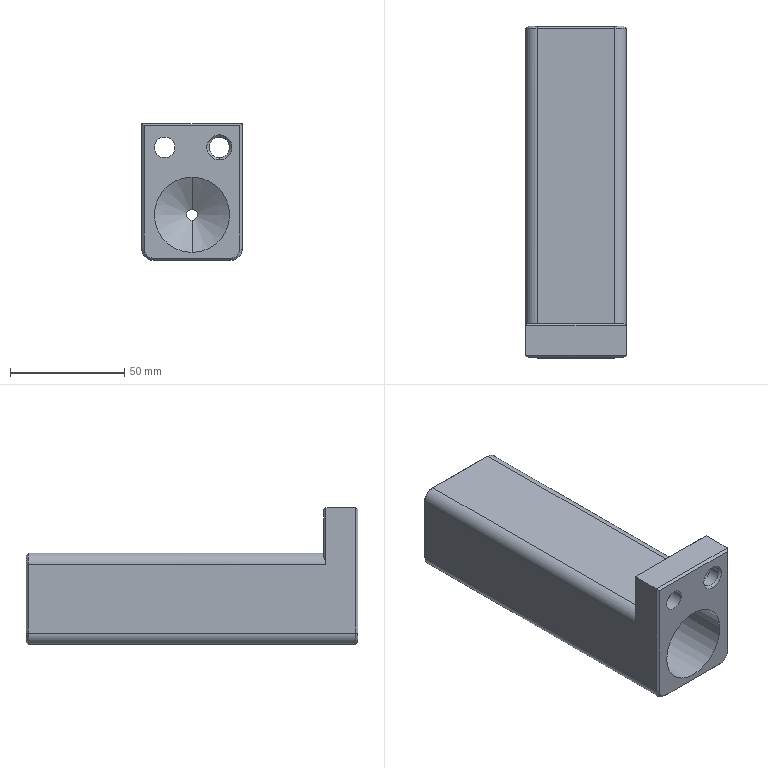Part | Creo | 1 solid | 45 faces | box 44 x 145.5 x 60 mm | volume 142551 mm3 | plane 21 | cylinder 14 | cone 10 | commonest cylinder face diameters 9 x4 10 x4 14 x4 33 x2
STEP:
#1=CARTESIAN_POINT('',(0.,0.,0.));
#2=DIRECTION('',(0.,0.,1.));
#3=DIRECTION('',(1.,0.,0.));
#4=AXIS2_PLACEMENT_3D('',#1,#2,#3);
#5=CARTESIAN_POINT('',(16.95,420.5,7.867));
#6=VERTEX_POINT('',#5);
#7=CARTESIAN_POINT('',(-17.05,420.5,7.867));
#8=VERTEX_POINT('',#7);
#9=CARTESIAN_POINT('',(16.95,420.5,7.867));
#10=DIRECTION('',(-1.,0.,0.));
#11=VECTOR('',#10,34.);
#12=LINE('',#9,#11);
#13=EDGE_CURVE('',#6,#8,#12,.T.);
#14=ORIENTED_EDGE('',*,*,#13,.T.);
#15=CARTESIAN_POINT('',(-21.05,420.5,3.866));
#16=VERTEX_POINT('',#15);
#17=CARTESIAN_POINT('',(-17.05,420.5,3.866));
#18=DIRECTION('',(0.,1.,0.));
#19=DIRECTION('',(-1.,0.,0.));
#20=AXIS2_PLACEMENT_3D('',#17,#18,#19);
#21=CIRCLE('',#20,4.);
#22=EDGE_CURVE('',#16,#8,#21,.T.);
#23=ORIENTED_EDGE('',*,*,#22,.F.);
#24=CARTESIAN_POINT('',(-21.05,420.5,-26.134));
#25=VERTEX_POINT('',#24);
#26=CARTESIAN_POINT('',(-21.05,420.5,3.866));
#27=DIRECTION('',(0.,0.,-1.));
#28=VECTOR('',#27,30.);
#29=LINE('',#26,#28);
#30=EDGE_CURVE('',#16,#25,#29,.T.);
#31=ORIENTED_EDGE('',*,*,#30,.T.);
#32=CARTESIAN_POINT('',(-17.05,420.5,-30.134));
#33=VERTEX_POINT('',#32);
#34=CARTESIAN_POINT('',(-17.05,420.5,-26.134));
#35=DIRECTION('',(0.,1.,0.));
#36=DIRECTION('',(0.,0.,-1.));
#37=AXIS2_PLACEMENT_3D('',#34,#35,#36);
#38=CIRCLE('',#37,4.);
#39=EDGE_CURVE('',#33,#25,#38,.T.);
#40=ORIENTED_EDGE('',*,*,#39,.F.);
#41=CARTESIAN_POINT('',(16.95,420.5,-30.134));
#42=VERTEX_POINT('',#41);
#43=CARTESIAN_POINT('',(-17.05,420.5,-30.134));
#44=DIRECTION('',(1.,0.,0.));
#45=VECTOR('',#44,34.);
#46=LINE('',#43,#45);
#47=EDGE_CURVE('',#33,#42,#46,.T.);
#48=ORIENTED_EDGE('',*,*,#47,.T.);
#49=CARTESIAN_POINT('',(20.95,420.5,-26.134));
#50=VERTEX_POINT('',#49);
#51=CARTESIAN_POINT('',(16.95,420.5,-26.134));
#52=DIRECTION('',(0.,1.,0.));
#53=DIRECTION('',(1.,0.,0.));
#54=AXIS2_PLACEMENT_3D('',#51,#52,#53);
#55=CIRCLE('',#54,4.);
#56=EDGE_CURVE('',#50,#42,#55,.T.);
#57=ORIENTED_EDGE('',*,*,#56,.F.);
#58=CARTESIAN_POINT('',(20.95,420.5,3.866));
#59=VERTEX_POINT('',#58);
#60=CARTESIAN_POINT('',(20.95,420.5,-26.134));
#61=DIRECTION('',(0.,0.,1.));
#62=VECTOR('',#61,30.);
#63=LINE('',#60,#62);
#64=EDGE_CURVE('',#50,#59,#63,.T.);
#65=ORIENTED_EDGE('',*,*,#64,.T.);
#66=CARTESIAN_POINT('',(16.95,420.5,3.866));
#67=DIRECTION('',(0.,1.,0.));
#68=DIRECTION('',(0.,0.,1.));
#69=AXIS2_PLACEMENT_3D('',#66,#67,#68);
#70=CIRCLE('',#69,4.);
#71=EDGE_CURVE('',#6,#59,#70,.T.);
#72=ORIENTED_EDGE('',*,*,#71,.F.);
#73=EDGE_LOOP('',(#14,#23,#31,#40,#48,#57,#65,#72));
#74=FACE_OUTER_BOUND('',#73,.F.);
#75=CARTESIAN_POINT('',(-0.05,420.5,-8.78));
#76=VERTEX_POINT('',#75);
#77=CARTESIAN_POINT('',(-0.05,420.5,-13.487));
#78=VERTEX_POINT('',#77);
#79=CARTESIAN_POINT('',(-0.05,420.5,-11.133));
#80=DIRECTION('',(0.,-1.,0.));
#81=DIRECTION('',(0.,0.,1.));
#82=AXIS2_PLACEMENT_3D('',#79,#80,#81);
#83=CIRCLE('',#82,2.354);
#84=EDGE_CURVE('',#76,#78,#83,.T.);
#85=ORIENTED_EDGE('',*,*,#84,.F.);
#86=CARTESIAN_POINT('',(-0.05,420.5,-11.133));
#87=DIRECTION('',(0.,-1.,0.));
#88=DIRECTION('',(0.,0.,-1.));
#89=AXIS2_PLACEMENT_3D('',#86,#87,#88);
#90=CIRCLE('',#89,2.354);
#91=EDGE_CURVE('',#78,#76,#90,.T.);
#92=ORIENTED_EDGE('',*,*,#91,.F.);
#93=EDGE_LOOP('',(#85,#92));
#94=FACE_BOUND('',#93,.F.);
#95=CARTESIAN_POINT('',(-0.05,420.5,-11.133));
#96=DIRECTION('',(0.,1.,0.));
#97=DIRECTION('',(0.,0.,1.));
#98=AXIS2_PLACEMENT_3D('',#95,#96,#97);
#99=PLANE('',#98);
#100=ADVANCED_FACE('',(#74,#94),#99,.T.);
#101=ORIENTED_EDGE('',*,*,#84,.T.);
#102=CARTESIAN_POINT('',(-0.05,412.,-27.634));
#103=VERTEX_POINT('',#102);
#104=CARTESIAN_POINT('',(-0.05,420.5,-13.487));
#105=DIRECTION('',(0.,-0.515,-0.8572));
#106=VECTOR('',#105,16.504);
#107=LINE('',#104,#106);
#108=EDGE_CURVE('',#78,#103,#107,.T.);
#109=ORIENTED_EDGE('',*,*,#108,.T.);
#110=CARTESIAN_POINT('',(-16.55,412.,-11.133));
#111=VERTEX_POINT('',#110);
#112=CARTESIAN_POINT('',(-0.05,412.,-11.133));
#113=DIRECTION('',(0.,-1.,0.));
#114=DIRECTION('',(-1.,0.,0.));
#115=AXIS2_PLACEMENT_3D('',#112,#113,#114);
#116=CIRCLE('',#115,16.5);
#117=EDGE_CURVE('',#111,#103,#116,.T.);
#118=ORIENTED_EDGE('',*,*,#117,.F.);
#119=CARTESIAN_POINT('',(-0.05,412.,5.367));
#120=VERTEX_POINT('',#119);
#121=CARTESIAN_POINT('',(-0.05,412.,-11.133));
#122=DIRECTION('',(0.,-1.,0.));
#123=DIRECTION('',(0.,0.,1.));
#124=AXIS2_PLACEMENT_3D('',#121,#122,#123);
#125=CIRCLE('',#124,16.5);
#126=EDGE_CURVE('',#120,#111,#125,.T.);
#127=ORIENTED_EDGE('',*,*,#126,.F.);
#128=CARTESIAN_POINT('',(-0.05,420.5,-8.78));
#129=DIRECTION('',(0.,-0.515,0.8572));
#130=VECTOR('',#129,16.504);
#131=LINE('',#128,#130);
#132=EDGE_CURVE('',#76,#120,#131,.T.);
#133=ORIENTED_EDGE('',*,*,#132,.F.);
#134=EDGE_LOOP('',(#101,#109,#118,#127,#133));
#135=FACE_OUTER_BOUND('',#134,.F.);
#136=CARTESIAN_POINT('',(-0.05,416.25,-11.133));
#137=DIRECTION('',(0.,-1.,0.));
#138=DIRECTION('',(0.,0.,-1.));
#139=AXIS2_PLACEMENT_3D('',#136,#137,#138);
#140=CONICAL_SURFACE('',#139,9.427,59.);
#141=ADVANCED_FACE('',(#135),#140,.F.);
#142=ORIENTED_EDGE('',*,*,#91,.T.);
#143=ORIENTED_EDGE('',*,*,#132,.T.);
#144=CARTESIAN_POINT('',(16.45,412.,-11.133));
#145=VERTEX_POINT('',#144);
#146=CARTESIAN_POINT('',(-0.05,412.,-11.133));
#147=DIRECTION('',(0.,-1.,0.));
#148=DIRECTION('',(1.,0.,0.));
#149=AXIS2_PLACEMENT_3D('',#146,#147,#148);
#150=CIRCLE('',#149,16.5);
#151=EDGE_CURVE('',#145,#120,#150,.T.);
#152=ORIENTED_EDGE('',*,*,#151,.F.);
#153=CARTESIAN_POINT('',(-0.05,412.,-11.133));
#154=DIRECTION('',(0.,-1.,0.));
#155=DIRECTION('',(0.,0.,-1.));
#156=AXIS2_PLACEMENT_3D('',#153,#154,#155);
#157=CIRCLE('',#156,16.5);
#158=EDGE_CURVE('',#103,#145,#157,.T.);
#159=ORIENTED_EDGE('',*,*,#158,.F.);
#160=ORIENTED_EDGE('',*,*,#108,.F.);
#161=EDGE_LOOP('',(#142,#143,#152,#159,#160));
#162=FACE_OUTER_BOUND('',#161,.F.);
#163=CARTESIAN_POINT('',(-0.05,416.25,-11.133));
#164=DIRECTION('',(0.,-1.,0.));
#165=DIRECTION('',(0.,0.,-1.));
#166=AXIS2_PLACEMENT_3D('',#163,#164,#165);
#167=CONICAL_SURFACE('',#166,9.427,59.);
#168=ADVANCED_FACE('',(#162),#167,.F.);
#169=CARTESIAN_POINT('',(-0.05,275.,5.367));
#170=VERTEX_POINT('',#169);
#171=CARTESIAN_POINT('',(16.45,275.,-11.133));
#172=VERTEX_POINT('',#171);
#173=CARTESIAN_POINT('',(-0.05,275.,-11.133));
#174=DIRECTION('',(0.,1.,0.));
#175=DIRECTION('',(0.,0.,1.));
#176=AXIS2_PLACEMENT_3D('',#173,#174,#175);
#177=CIRCLE('',#176,16.5);
#178=EDGE_CURVE('',#170,#172,#177,.T.);
#179=ORIENTED_EDGE('',*,*,#178,.T.);
#180=CARTESIAN_POINT('',(16.45,412.,-11.133));
#181=DIRECTION('',(0.,-1.,0.));
#182=VECTOR('',#181,137.);
#183=LINE('',#180,#182);
#184=EDGE_CURVE('',#145,#172,#183,.T.);
#185=ORIENTED_EDGE('',*,*,#184,.F.);
#186=ORIENTED_EDGE('',*,*,#151,.T.);
#187=ORIENTED_EDGE('',*,*,#126,.T.);
#188=CARTESIAN_POINT('',(-16.55,275.,-11.133));
#189=VERTEX_POINT('',#188);
#190=CARTESIAN_POINT('',(-16.55,412.,-11.133));
#191=DIRECTION('',(0.,-1.,0.));
#192=VECTOR('',#191,137.);
#193=LINE('',#190,#192);
#194=EDGE_CURVE('',#111,#189,#193,.T.);
#195=ORIENTED_EDGE('',*,*,#194,.T.);
#196=CARTESIAN_POINT('',(-0.05,275.,-11.133));
#197=DIRECTION('',(0.,1.,0.));
#198=DIRECTION('',(-1.,0.,0.));
#199=AXIS2_PLACEMENT_3D('',#196,#197,#198);
#200=CIRCLE('',#199,16.5);
#201=EDGE_CURVE('',#189,#170,#200,.T.);
#202=ORIENTED_EDGE('',*,*,#201,.T.);
#203=EDGE_LOOP('',(#179,#185,#186,#187,#195,#202));
#204=FACE_OUTER_BOUND('',#203,.F.);
#205=CARTESIAN_POINT('',(-0.05,375.5,-11.133));
#206=DIRECTION('',(0.,-1.,0.));
#207=DIRECTION('',(-1.,0.,0.));
#208=AXIS2_PLACEMENT_3D('',#205,#206,#207);
#209=CYLINDRICAL_SURFACE('',#208,16.5);
#210=ADVANCED_FACE('',(#204),#209,.F.);
#211=CARTESIAN_POINT('',(-21.05,275.,27.866));
#212=VERTEX_POINT('',#211);
#213=CARTESIAN_POINT('',(20.95,275.,27.866));
#214=VERTEX_POINT('',#213);
#215=CARTESIAN_POINT('',(-21.05,275.,27.866));
#216=DIRECTION('',(1.,0.,0.));
#217=VECTOR('',#216,42.);
#218=LINE('',#215,#217);
#219=EDGE_CURVE('',#212,#214,#218,.T.);
#220=ORIENTED_EDGE('',*,*,#219,.T.);
#221=CARTESIAN_POINT('',(20.95,275.,-26.134));
#222=VERTEX_POINT('',#221);
#223=CARTESIAN_POINT('',(20.95,275.,27.866));
#224=DIRECTION('',(0.,0.,-1.));
#225=VECTOR('',#224,54.);
#226=LINE('',#223,#225);
#227=EDGE_CURVE('',#214,#222,#226,.T.);
#228=ORIENTED_EDGE('',*,*,#227,.T.);
#229=CARTESIAN_POINT('',(16.95,275.,-30.134));
#230=VERTEX_POINT('',#229);
#231=CARTESIAN_POINT('',(16.95,275.,-26.134));
#232=DIRECTION('',(0.,-1.,0.));
#233=DIRECTION('',(0.,0.,-1.));
#234=AXIS2_PLACEMENT_3D('',#231,#232,#233);
#235=CIRCLE('',#234,4.);
#236=EDGE_CURVE('',#230,#222,#235,.T.);
#237=ORIENTED_EDGE('',*,*,#236,.F.);
#238=CARTESIAN_POINT('',(-17.05,275.,-30.134));
#239=VERTEX_POINT('',#238);
#240=CARTESIAN_POINT('',(16.95,275.,-30.134));
#241=DIRECTION('',(-1.,0.,0.));
#242=VECTOR('',#241,34.);
#243=LINE('',#240,#242);
#244=EDGE_CURVE('',#230,#239,#243,.T.);
#245=ORIENTED_EDGE('',*,*,#244,.T.);
#246=CARTESIAN_POINT('',(-21.05,275.,-26.134));
#247=VERTEX_POINT('',#246);
#248=CARTESIAN_POINT('',(-17.05,275.,-26.134));
#249=DIRECTION('',(0.,-1.,0.));
#250=DIRECTION('',(-1.,0.,0.));
#251=AXIS2_PLACEMENT_3D('',#248,#249,#250);
#252=CIRCLE('',#251,4.);
#253=EDGE_CURVE('',#247,#239,#252,.T.);
#254=ORIENTED_EDGE('',*,*,#253,.F.);
#255=CARTESIAN_POINT('',(-21.05,275.,-26.134));
#256=DIRECTION('',(0.,0.,1.));
#257=VECTOR('',#256,54.);
#258=LINE('',#255,#257);
#259=EDGE_CURVE('',#247,#212,#258,.T.);
#260=ORIENTED_EDGE('',*,*,#259,.T.);
#261=EDGE_LOOP('',(#220,#228,#237,#245,#254,#260));
#262=FACE_OUTER_BOUND('',#261,.F.);
#263=CARTESIAN_POINT('',(11.95,275.,12.92));
#264=VERTEX_POINT('',#263);
#265=CARTESIAN_POINT('',(11.95,275.,23.92));
#266=VERTEX_POINT('',#265);
#267=CARTESIAN_POINT('',(11.95,275.,18.42));
#268=DIRECTION('',(0.,1.,0.));
#269=DIRECTION('',(0.,0.,-1.));
#270=AXIS2_PLACEMENT_3D('',#267,#268,#269);
#271=CIRCLE('',#270,5.5);
#272=EDGE_CURVE('',#264,#266,#271,.T.);
#273=ORIENTED_EDGE('',*,*,#272,.F.);
#274=CARTESIAN_POINT('',(11.95,275.,18.42));
#275=DIRECTION('',(0.,1.,0.));
#276=DIRECTION('',(0.,0.,1.));
#277=AXIS2_PLACEMENT_3D('',#274,#275,#276);
#278=CIRCLE('',#277,5.5);
#279=EDGE_CURVE('',#266,#264,#278,.T.);
#280=ORIENTED_EDGE('',*,*,#279,.F.);
#281=EDGE_LOOP('',(#273,#280));
#282=FACE_BOUND('',#281,.F.);
#283=CARTESIAN_POINT('',(-0.05,275.,-27.634));
#284=VERTEX_POINT('',#283);
#285=CARTESIAN_POINT('',(-0.05,275.,-11.133));
#286=DIRECTION('',(0.,1.,0.));
#287=DIRECTION('',(0.,0.,-1.));
#288=AXIS2_PLACEMENT_3D('',#285,#286,#287);
#289=CIRCLE('',#288,16.5);
#290=EDGE_CURVE('',#284,#189,#289,.T.);
#291=ORIENTED_EDGE('',*,*,#290,.F.);
#292=CARTESIAN_POINT('',(-0.05,275.,-11.133));
#293=DIRECTION('',(0.,1.,0.));
#294=DIRECTION('',(1.,0.,0.));
#295=AXIS2_PLACEMENT_3D('',#292,#293,#294);
#296=CIRCLE('',#295,16.5);
#297=EDGE_CURVE('',#172,#284,#296,.T.);
#298=ORIENTED_EDGE('',*,*,#297,.F.);
#299=ORIENTED_EDGE('',*,*,#178,.F.);
#300=ORIENTED_EDGE('',*,*,#201,.F.);
#301=EDGE_LOOP('',(#291,#298,#299,#300));
#302=FACE_BOUND('',#301,.F.);
#303=CARTESIAN_POINT('',(-7.55,275.,18.42));
#304=VERTEX_POINT('',#303);
#305=CARTESIAN_POINT('',(-16.55,275.,18.42));
#306=VERTEX_POINT('',#305);
#307=CARTESIAN_POINT('',(-12.05,275.,18.42));
#308=DIRECTION('',(0.,1.,0.));
#309=DIRECTION('',(1.,0.,0.));
#310=AXIS2_PLACEMENT_3D('',#307,#308,#309);
#311=CIRCLE('',#310,4.5);
#312=EDGE_CURVE('',#304,#306,#311,.T.);
#313=ORIENTED_EDGE('',*,*,#312,.F.);
#314=CARTESIAN_POINT('',(-12.05,275.,18.42));
#315=DIRECTION('',(0.,1.,0.));
#316=DIRECTION('',(-1.,0.,0.));
#317=AXIS2_PLACEMENT_3D('',#314,#315,#316);
#318=CIRCLE('',#317,4.5);
#319=EDGE_CURVE('',#306,#304,#318,.T.);
#320=ORIENTED_EDGE('',*,*,#319,.F.);
#321=EDGE_LOOP('',(#313,#320));
#322=FACE_BOUND('',#321,.F.);
#323=CARTESIAN_POINT('',(0.,275.,0.));
#324=DIRECTION('',(0.,-1.,0.));
#325=DIRECTION('',(0.,0.,-1.));
#326=AXIS2_PLACEMENT_3D('',#323,#324,#325);
#327=PLANE('',#326);
#328=ADVANCED_FACE('',(#262,#282,#302,#322),#327,.T.);
#329=CARTESIAN_POINT('',(11.95,276.,13.92));
#330=VERTEX_POINT('',#329);
#331=CARTESIAN_POINT('',(7.45,276.,18.42));
#332=VERTEX_POINT('',#331);
#333=CARTESIAN_POINT('',(11.95,276.,18.42));
#334=DIRECTION('',(0.,1.,0.));
#335=DIRECTION('',(0.,0.,-1.));
#336=AXIS2_PLACEMENT_3D('',#333,#334,#335);
#337=CIRCLE('',#336,4.5);
#338=EDGE_CURVE('',#330,#332,#337,.T.);
#339=ORIENTED_EDGE('',*,*,#338,.F.);
#340=CARTESIAN_POINT('',(11.95,276.,13.92));
#341=DIRECTION('',(0.,-0.7071,-0.7071));
#342=VECTOR('',#341,1.414);
#343=LINE('',#340,#342);
#344=EDGE_CURVE('',#330,#264,#343,.T.);
#345=ORIENTED_EDGE('',*,*,#344,.T.);
#346=ORIENTED_EDGE('',*,*,#272,.T.);
#347=CARTESIAN_POINT('',(11.95,276.,22.92));
#348=VERTEX_POINT('',#347);
#349=CARTESIAN_POINT('',(11.95,276.,22.92));
#350=DIRECTION('',(0.,-0.7071,0.7071));
#351=VECTOR('',#350,1.414);
#352=LINE('',#349,#351);
#353=EDGE_CURVE('',#348,#266,#352,.T.);
#354=ORIENTED_EDGE('',*,*,#353,.F.);
#355=CARTESIAN_POINT('',(11.95,276.,18.42));
#356=DIRECTION('',(0.,1.,0.));
#357=DIRECTION('',(-1.,0.,0.));
#358=AXIS2_PLACEMENT_3D('',#355,#356,#357);
#359=CIRCLE('',#358,4.5);
#360=EDGE_CURVE('',#332,#348,#359,.T.);
#361=ORIENTED_EDGE('',*,*,#360,.F.);
#362=EDGE_LOOP('',(#339,#345,#346,#354,#361));
#363=FACE_OUTER_BOUND('',#362,.F.);
#364=CARTESIAN_POINT('',(11.95,275.5,18.42));
#365=DIRECTION('',(0.,-1.,0.));
#366=DIRECTION('',(0.,0.,-1.));
#367=AXIS2_PLACEMENT_3D('',#364,#365,#366);
#368=CONICAL_SURFACE('',#367,5.,45.);
#369=ADVANCED_FACE('',(#363),#368,.F.);
#370=CARTESIAN_POINT('',(16.45,276.,18.42));
#371=VERTEX_POINT('',#370);
#372=CARTESIAN_POINT('',(11.95,276.,18.42));
#373=DIRECTION('',(0.,1.,0.));
#374=DIRECTION('',(1.,0.,0.));
#375=AXIS2_PLACEMENT_3D('',#372,#373,#374);
#376=CIRCLE('',#375,4.5);
#377=EDGE_CURVE('',#371,#330,#376,.T.);
#378=ORIENTED_EDGE('',*,*,#377,.T.);
#379=ORIENTED_EDGE('',*,*,#338,.T.);
#380=CARTESIAN_POINT('',(7.45,281.,18.42));
#381=VERTEX_POINT('',#380);
#382=CARTESIAN_POINT('',(7.45,276.,18.42));
#383=DIRECTION('',(0.,1.,0.));
#384=VECTOR('',#383,5.);
#385=LINE('',#382,#384);
#386=EDGE_CURVE('',#332,#381,#385,.T.);
#387=ORIENTED_EDGE('',*,*,#386,.T.);
#388=CARTESIAN_POINT('',(16.45,281.,18.42));
#389=VERTEX_POINT('',#388);
#390=CARTESIAN_POINT('',(11.95,281.,18.42));
#391=DIRECTION('',(0.,-1.,0.));
#392=DIRECTION('',(-1.,0.,0.));
#393=AXIS2_PLACEMENT_3D('',#390,#391,#392);
#394=CIRCLE('',#393,4.5);
#395=EDGE_CURVE('',#381,#389,#394,.T.);
#396=ORIENTED_EDGE('',*,*,#395,.T.);
#397=CARTESIAN_POINT('',(16.45,276.,18.42));
#398=DIRECTION('',(0.,1.,0.));
#399=VECTOR('',#398,5.);
#400=LINE('',#397,#399);
#401=EDGE_CURVE('',#371,#389,#400,.T.);
#402=ORIENTED_EDGE('',*,*,#401,.F.);
#403=EDGE_LOOP('',(#378,#379,#387,#396,#402));
#404=FACE_OUTER_BOUND('',#403,.F.);
#405=CARTESIAN_POINT('',(11.95,290.,18.42));
#406=DIRECTION('',(0.,1.,0.));
#407=DIRECTION('',(1.,0.,0.));
#408=AXIS2_PLACEMENT_3D('',#405,#406,#407);
#409=CYLINDRICAL_SURFACE('',#408,4.5);
#410=ADVANCED_FACE('',(#404),#409,.F.);
#411=CARTESIAN_POINT('',(11.95,276.,18.42));
#412=DIRECTION('',(0.,1.,0.));
#413=DIRECTION('',(0.,0.,1.));
#414=AXIS2_PLACEMENT_3D('',#411,#412,#413);
#415=CIRCLE('',#414,4.5);
#416=EDGE_CURVE('',#348,#371,#415,.T.);
#417=ORIENTED_EDGE('',*,*,#416,.F.);
#418=ORIENTED_EDGE('',*,*,#353,.T.);
#419=ORIENTED_EDGE('',*,*,#279,.T.);
#420=ORIENTED_EDGE('',*,*,#344,.F.);
#421=ORIENTED_EDGE('',*,*,#377,.F.);
#422=EDGE_LOOP('',(#417,#418,#419,#420,#421));
#423=FACE_OUTER_BOUND('',#422,.F.);
#424=CARTESIAN_POINT('',(11.95,275.5,18.42));
#425=DIRECTION('',(0.,-1.,0.));
#426=DIRECTION('',(0.,0.,-1.));
#427=AXIS2_PLACEMENT_3D('',#424,#425,#426);
#428=CONICAL_SURFACE('',#427,5.,45.);
#429=ADVANCED_FACE('',(#423),#428,.F.);
#430=ORIENTED_EDGE('',*,*,#416,.T.);
#431=ORIENTED_EDGE('',*,*,#401,.T.);
#432=CARTESIAN_POINT('',(11.95,281.,18.42));
#433=DIRECTION('',(0.,-1.,0.));
#434=DIRECTION('',(1.,0.,0.));
#435=AXIS2_PLACEMENT_3D('',#432,#433,#434);
#436=CIRCLE('',#435,4.5);
#437=EDGE_CURVE('',#389,#381,#436,.T.);
#438=ORIENTED_EDGE('',*,*,#437,.T.);
#439=ORIENTED_EDGE('',*,*,#386,.F.);
#440=ORIENTED_EDGE('',*,*,#360,.T.);
#441=EDGE_LOOP('',(#430,#431,#438,#439,#440));
#442=FACE_OUTER_BOUND('',#441,.F.);
#443=CARTESIAN_POINT('',(11.95,290.,18.42));
#444=DIRECTION('',(0.,1.,0.));
#445=DIRECTION('',(1.,0.,0.));
#446=AXIS2_PLACEMENT_3D('',#443,#444,#445);
#447=CYLINDRICAL_SURFACE('',#446,4.5);
#448=ADVANCED_FACE('',(#442),#447,.F.);
#449=CARTESIAN_POINT('',(18.95,281.,18.42));
#450=VERTEX_POINT('',#449);
#451=CARTESIAN_POINT('',(4.95,281.,18.42));
#452=VERTEX_POINT('',#451);
#453=CARTESIAN_POINT('',(11.95,281.,18.42));
#454=DIRECTION('',(0.,1.,0.));
#455=DIRECTION('',(1.,0.,0.));
#456=AXIS2_PLACEMENT_3D('',#453,#454,#455);
#457=CIRCLE('',#456,7.);
#458=EDGE_CURVE('',#450,#452,#457,.T.);
#459=ORIENTED_EDGE('',*,*,#458,.F.);
#460=CARTESIAN_POINT('',(11.95,281.,18.42));
#461=DIRECTION('',(0.,1.,0.));
#462=DIRECTION('',(-1.,0.,0.));
#463=AXIS2_PLACEMENT_3D('',#460,#461,#462);
#464=CIRCLE('',#463,7.);
#465=EDGE_CURVE('',#452,#450,#464,.T.);
#466=ORIENTED_EDGE('',*,*,#465,.F.);
#467=EDGE_LOOP('',(#459,#466));
#468=FACE_OUTER_BOUND('',#467,.F.);
#469=ORIENTED_EDGE('',*,*,#437,.F.);
#470=ORIENTED_EDGE('',*,*,#395,.F.);
#471=EDGE_LOOP('',(#469,#470));
#472=FACE_BOUND('',#471,.F.);
#473=CARTESIAN_POINT('',(11.95,281.,11.42));
#474=DIRECTION('',(0.,-1.,0.));
#475=DIRECTION('',(-1.,0.,0.));
#476=AXIS2_PLACEMENT_3D('',#473,#474,#475);
#477=PLANE('',#476);
#478=ADVANCED_FACE('',(#468,#472),#477,.F.);
#479=ORIENTED_EDGE('',*,*,#458,.T.);
#480=CARTESIAN_POINT('',(4.95,290.,18.42));
#481=VERTEX_POINT('',#480);
#482=CARTESIAN_POINT('',(4.95,281.,18.42));
#483=DIRECTION('',(0.,1.,0.));
#484=VECTOR('',#483,9.);
#485=LINE('',#482,#484);
#486=EDGE_CURVE('',#452,#481,#485,.T.);
#487=ORIENTED_EDGE('',*,*,#486,.T.);
#488=CARTESIAN_POINT('',(18.95,290.,18.42));
#489=VERTEX_POINT('',#488);
#490=CARTESIAN_POINT('',(11.95,290.,18.42));
#491=DIRECTION('',(0.,-1.,0.));
#492=DIRECTION('',(-1.,0.,0.));
#493=AXIS2_PLACEMENT_3D('',#490,#491,#492);
#494=CIRCLE('',#493,7.);
#495=EDGE_CURVE('',#481,#489,#494,.T.);
#496=ORIENTED_EDGE('',*,*,#495,.T.);
#497=CARTESIAN_POINT('',(18.95,281.,18.42));
#498=DIRECTION('',(0.,1.,0.));
#499=VECTOR('',#498,9.);
#500=LINE('',#497,#499);
#501=EDGE_CURVE('',#450,#489,#500,.T.);
#502=ORIENTED_EDGE('',*,*,#501,.F.);
#503=EDGE_LOOP('',(#479,#487,#496,#502));
#504=FACE_OUTER_BOUND('',#503,.F.);
#505=CARTESIAN_POINT('',(11.95,290.,18.42));
#506=DIRECTION('',(0.,1.,0.));
#507=DIRECTION('',(1.,0.,0.));
#508=AXIS2_PLACEMENT_3D('',#505,#506,#507);
#509=CYLINDRICAL_SURFACE('',#508,7.);
#510=ADVANCED_FACE('',(#504),#509,.F.);
#511=ORIENTED_EDGE('',*,*,#465,.T.);
#512=ORIENTED_EDGE('',*,*,#501,.T.);
#513=CARTESIAN_POINT('',(11.95,290.,18.42));
#514=DIRECTION('',(0.,-1.,0.));
#515=DIRECTION('',(1.,0.,0.));
#516=AXIS2_PLACEMENT_3D('',#513,#514,#515);
#517=CIRCLE('',#516,7.);
#518=EDGE_CURVE('',#489,#481,#517,.T.);
#519=ORIENTED_EDGE('',*,*,#518,.T.);
#520=ORIENTED_EDGE('',*,*,#486,.F.);
#521=EDGE_LOOP('',(#511,#512,#519,#520));
#522=FACE_OUTER_BOUND('',#521,.F.);
#523=CARTESIAN_POINT('',(11.95,290.,18.42));
#524=DIRECTION('',(0.,1.,0.));
#525=DIRECTION('',(1.,0.,0.));
#526=AXIS2_PLACEMENT_3D('',#523,#524,#525);
#527=CYLINDRICAL_SURFACE('',#526,7.);
#528=ADVANCED_FACE('',(#522),#527,.F.);
#529=CARTESIAN_POINT('',(-17.05,290.,8.867));
#530=VERTEX_POINT('',#529);
#531=CARTESIAN_POINT('',(-21.05,290.,6.867));
#532=VERTEX_POINT('',#531);
#533=CARTESIAN_POINT('',(-17.05,290.,3.866));
#534=DIRECTION('',(0.,-1.,0.));
#535=DIRECTION('',(0.,0.,1.));
#536=AXIS2_PLACEMENT_3D('',#533,#534,#535);
#537=CIRCLE('',#536,5.);
#538=EDGE_CURVE('',#530,#532,#537,.T.);
#539=ORIENTED_EDGE('',*,*,#538,.F.);
#540=CARTESIAN_POINT('',(16.95,290.,8.867));
#541=VERTEX_POINT('',#540);
#542=CARTESIAN_POINT('',(16.95,290.,8.867));
#543=DIRECTION('',(-1.,0.,0.));
#544=VECTOR('',#543,34.);
#545=LINE('',#542,#544);
#546=EDGE_CURVE('',#541,#530,#545,.T.);
#547=ORIENTED_EDGE('',*,*,#546,.F.);
#548=CARTESIAN_POINT('',(20.95,290.,6.867));
#549=VERTEX_POINT('',#548);
#550=CARTESIAN_POINT('',(16.95,290.,3.866));
#551=DIRECTION('',(0.,-1.,0.));
#552=DIRECTION('',(0.8,0.,0.6));
#553=AXIS2_PLACEMENT_3D('',#550,#551,#552);
#554=CIRCLE('',#553,5.);
#555=EDGE_CURVE('',#549,#541,#554,.T.);
#556=ORIENTED_EDGE('',*,*,#555,.F.);
#557=CARTESIAN_POINT('',(20.95,290.,27.866));
#558=VERTEX_POINT('',#557);
#559=CARTESIAN_POINT('',(20.95,290.,6.867));
#560=DIRECTION('',(0.,0.,1.));
#561=VECTOR('',#560,21.);
#562=LINE('',#559,#561);
#563=EDGE_CURVE('',#549,#558,#562,.T.);
#564=ORIENTED_EDGE('',*,*,#563,.T.);
#565=CARTESIAN_POINT('',(-21.05,290.,27.866));
#566=VERTEX_POINT('',#565);
#567=CARTESIAN_POINT('',(20.95,290.,27.866));
#568=DIRECTION('',(-1.,0.,0.));
#569=VECTOR('',#568,42.);
#570=LINE('',#567,#569);
#571=EDGE_CURVE('',#558,#566,#570,.T.);
#572=ORIENTED_EDGE('',*,*,#571,.T.);
#573=CARTESIAN_POINT('',(-21.05,290.,27.866));
#574=DIRECTION('',(0.,0.,-1.));
#575=VECTOR('',#574,21.);
#576=LINE('',#573,#575);
#577=EDGE_CURVE('',#566,#532,#576,.T.);
#578=ORIENTED_EDGE('',*,*,#577,.T.);
#579=EDGE_LOOP('',(#539,#547,#556,#564,#572,#578));
#580=FACE_OUTER_BOUND('',#579,.F.);
#581=ORIENTED_EDGE('',*,*,#518,.F.);
#582=ORIENTED_EDGE('',*,*,#495,.F.);
#583=EDGE_LOOP('',(#581,#582));
#584=FACE_BOUND('',#583,.F.);
#585=CARTESIAN_POINT('',(-5.05,290.,18.42));
#586=VERTEX_POINT('',#585);
#587=CARTESIAN_POINT('',(-19.05,290.,18.42));
#588=VERTEX_POINT('',#587);
#589=CARTESIAN_POINT('',(-12.05,290.,18.42));
#590=DIRECTION('',(0.,-1.,0.));
#591=DIRECTION('',(1.,0.,0.));
#592=AXIS2_PLACEMENT_3D('',#589,#590,#591);
#593=CIRCLE('',#592,7.);
#594=EDGE_CURVE('',#586,#588,#593,.T.);
#595=ORIENTED_EDGE('',*,*,#594,.F.);
#596=CARTESIAN_POINT('',(-12.05,290.,18.42));
#597=DIRECTION('',(0.,-1.,0.));
#598=DIRECTION('',(-1.,0.,0.));
#599=AXIS2_PLACEMENT_3D('',#596,#597,#598);
#600=CIRCLE('',#599,7.);
#601=EDGE_CURVE('',#588,#586,#600,.T.);
#602=ORIENTED_EDGE('',*,*,#601,.F.);
#603=EDGE_LOOP('',(#595,#602));
#604=FACE_BOUND('',#603,.F.);
#605=CARTESIAN_POINT('',(21.95,290.,28.866));
#606=DIRECTION('',(0.,1.,0.));
#607=DIRECTION('',(0.,0.,1.));
#608=AXIS2_PLACEMENT_3D('',#605,#606,#607);
#609=PLANE('',#608);
#610=ADVANCED_FACE('',(#580,#584,#604),#609,.T.);
#611=CARTESIAN_POINT('',(-17.05,419.5,8.867));
#612=VERTEX_POINT('',#611);
#613=CARTESIAN_POINT('',(-17.05,290.,8.867));
#614=DIRECTION('',(0.,1.,0.));
#615=VECTOR('',#614,129.5);
#616=LINE('',#613,#615);
#617=EDGE_CURVE('',#530,#612,#616,.T.);
#618=ORIENTED_EDGE('',*,*,#617,.F.);
#619=ORIENTED_EDGE('',*,*,#538,.T.);
#620=CARTESIAN_POINT('',(-22.05,289.,3.866));
#621=VERTEX_POINT('',#620);
#622=CARTESIAN_POINT('',(-22.05,289.,3.866));
#623=CARTESIAN_POINT('',(-22.05,289.,4.468));
#624=CARTESIAN_POINT('',(-21.844,289.206,5.546));
#625=CARTESIAN_POINT('',(-21.36,289.69,6.454));
#626=CARTESIAN_POINT('',(-21.05,290.,6.867));
#627=B_SPLINE_CURVE_WITH_KNOTS('',3,(#622,#623,#624,#625,#626),.UNSPECIFIED.,.F.,.F.,(4,1,4),(0.,0.5,1.),.UNSPECIFIED.);
#628=EDGE_CURVE('',#621,#532,#627,.T.);
#629=ORIENTED_EDGE('',*,*,#628,.F.);
#630=CARTESIAN_POINT('',(-22.05,419.5,3.866));
#631=VERTEX_POINT('',#630);
#632=CARTESIAN_POINT('',(-22.05,419.5,3.866));
#633=DIRECTION('',(0.,-1.,0.));
#634=VECTOR('',#633,130.5);
#635=LINE('',#632,#634);
#636=EDGE_CURVE('',#631,#621,#635,.T.);
#637=ORIENTED_EDGE('',*,*,#636,.F.);
#638=CARTESIAN_POINT('',(-17.05,419.5,3.866));
#639=DIRECTION('',(0.,1.,0.));
#640=DIRECTION('',(-1.,0.,0.));
#641=AXIS2_PLACEMENT_3D('',#638,#639,#640);
#642=CIRCLE('',#641,5.);
#643=EDGE_CURVE('',#631,#612,#642,.T.);
#644=ORIENTED_EDGE('',*,*,#643,.T.);
#645=EDGE_LOOP('',(#618,#619,#629,#637,#644));
#646=FACE_OUTER_BOUND('',#645,.F.);
#647=CARTESIAN_POINT('',(-17.05,420.5,3.866));
#648=DIRECTION('',(0.,-1.,0.));
#649=DIRECTION('',(0.,0.,-1.));
#650=AXIS2_PLACEMENT_3D('',#647,#648,#649);
#651=CYLINDRICAL_SURFACE('',#650,5.);
#652=ADVANCED_FACE('',(#646),#651,.T.);
#653=CARTESIAN_POINT('',(16.95,419.5,8.867));
#654=VERTEX_POINT('',#653);
#655=CARTESIAN_POINT('',(16.95,419.5,8.867));
#656=DIRECTION('',(0.,-1.,0.));
#657=VECTOR('',#656,129.5);
#658=LINE('',#655,#657);
#659=EDGE_CURVE('',#654,#541,#658,.T.);
#660=ORIENTED_EDGE('',*,*,#659,.T.);
#661=ORIENTED_EDGE('',*,*,#546,.T.);
#662=ORIENTED_EDGE('',*,*,#617,.T.);
#663=CARTESIAN_POINT('',(-17.05,419.5,8.867));
#664=DIRECTION('',(1.,0.,0.));
#665=VECTOR('',#664,34.);
#666=LINE('',#663,#665);
#667=EDGE_CURVE('',#612,#654,#666,.T.);
#668=ORIENTED_EDGE('',*,*,#667,.T.);
#669=EDGE_LOOP('',(#660,#661,#662,#668));
#670=FACE_OUTER_BOUND('',#669,.F.);
#671=CARTESIAN_POINT('',(-0.05,420.5,8.867));
#672=DIRECTION('',(0.,0.,1.));
#673=DIRECTION('',(1.,0.,0.));
#674=AXIS2_PLACEMENT_3D('',#671,#672,#673);
#675=PLANE('',#674);
#676=ADVANCED_FACE('',(#670),#675,.T.);
#677=CARTESIAN_POINT('',(21.95,289.,3.866));
#678=VERTEX_POINT('',#677);
#679=CARTESIAN_POINT('',(21.95,419.5,3.866));
#680=VERTEX_POINT('',#679);
#681=CARTESIAN_POINT('',(21.95,289.,3.866));
#682=DIRECTION('',(0.,1.,0.));
#683=VECTOR('',#682,130.5);
#684=LINE('',#681,#683);
#685=EDGE_CURVE('',#678,#680,#684,.T.);
#686=ORIENTED_EDGE('',*,*,#685,.F.);
#687=CARTESIAN_POINT('',(21.95,289.,3.866));
#688=CARTESIAN_POINT('',(21.95,289.,4.468));
#689=CARTESIAN_POINT('',(21.744,289.206,5.546));
#690=CARTESIAN_POINT('',(21.26,289.69,6.454));
#691=CARTESIAN_POINT('',(20.95,290.,6.867));
#692=B_SPLINE_CURVE_WITH_KNOTS('',3,(#687,#688,#689,#690,#691),.UNSPECIFIED.,.F.,.F.,(4,1,4),(0.,0.5,1.),.UNSPECIFIED.);
#693=EDGE_CURVE('',#678,#549,#692,.T.);
#694=ORIENTED_EDGE('',*,*,#693,.T.);
#695=ORIENTED_EDGE('',*,*,#555,.T.);
#696=ORIENTED_EDGE('',*,*,#659,.F.);
#697=CARTESIAN_POINT('',(16.95,419.5,3.866));
#698=DIRECTION('',(0.,1.,0.));
#699=DIRECTION('',(0.,0.,1.));
#700=AXIS2_PLACEMENT_3D('',#697,#698,#699);
#701=CIRCLE('',#700,5.);
#702=EDGE_CURVE('',#654,#680,#701,.T.);
#703=ORIENTED_EDGE('',*,*,#702,.T.);
#704=EDGE_LOOP('',(#686,#694,#695,#696,#703));
#705=FACE_OUTER_BOUND('',#704,.F.);
#706=CARTESIAN_POINT('',(16.95,420.5,3.866));
#707=DIRECTION('',(0.,1.,0.));
#708=DIRECTION('',(0.,0.,1.));
#709=AXIS2_PLACEMENT_3D('',#706,#707,#708);
#710=CYLINDRICAL_SURFACE('',#709,5.);
#711=ADVANCED_FACE('',(#705),#710,.T.);
#712=ORIENTED_EDGE('',*,*,#685,.T.);
#713=CARTESIAN_POINT('',(21.95,419.5,-26.134));
#714=VERTEX_POINT('',#713);
#715=CARTESIAN_POINT('',(21.95,419.5,3.866));
#716=DIRECTION('',(0.,0.,-1.));
#717=VECTOR('',#716,30.);
#718=LINE('',#715,#717);
#719=EDGE_CURVE('',#680,#714,#718,.T.);
#720=ORIENTED_EDGE('',*,*,#719,.T.);
#721=CARTESIAN_POINT('',(21.95,276.,-26.134));
#722=VERTEX_POINT('',#721);
#723=CARTESIAN_POINT('',(21.95,419.5,-26.134));
#724=DIRECTION('',(0.,-1.,0.));
#725=VECTOR('',#724,143.5);
#726=LINE('',#723,#725);
#727=EDGE_CURVE('',#714,#722,#726,.T.);
#728=ORIENTED_EDGE('',*,*,#727,.T.);
#729=CARTESIAN_POINT('',(21.95,276.,28.866));
#730=VERTEX_POINT('',#729);
#731=CARTESIAN_POINT('',(21.95,276.,-26.134));
#732=DIRECTION('',(0.,0.,1.));
#733=VECTOR('',#732,55.);
#734=LINE('',#731,#733);
#735=EDGE_CURVE('',#722,#730,#734,.T.);
#736=ORIENTED_EDGE('',*,*,#735,.T.);
#737=CARTESIAN_POINT('',(21.95,289.,28.866));
#738=VERTEX_POINT('',#737);
#739=CARTESIAN_POINT('',(21.95,276.,28.866));
#740=DIRECTION('',(0.,1.,0.));
#741=VECTOR('',#740,13.);
#742=LINE('',#739,#741);
#743=EDGE_CURVE('',#730,#738,#742,.T.);
#744=ORIENTED_EDGE('',*,*,#743,.T.);
#745=CARTESIAN_POINT('',(21.95,289.,28.866));
#746=DIRECTION('',(0.,0.,-1.));
#747=VECTOR('',#746,25.);
#748=LINE('',#745,#747);
#749=EDGE_CURVE('',#738,#678,#748,.T.);
#750=ORIENTED_EDGE('',*,*,#749,.T.);
#751=EDGE_LOOP('',(#712,#720,#728,#736,#744,#750));
#752=FACE_OUTER_BOUND('',#751,.F.);
#753=CARTESIAN_POINT('',(21.95,282.,-6.133));
#754=DIRECTION('',(1.,0.,0.));
#755=DIRECTION('',(0.,0.,-1.));
#756=AXIS2_PLACEMENT_3D('',#753,#754,#755);
#757=PLANE('',#756);
#758=ADVANCED_FACE('',(#752),#757,.T.);
#759=CARTESIAN_POINT('',(20.95,420.5,-26.134));
#760=DIRECTION('',(0.7071,-0.7071,0.));
#761=VECTOR('',#760,1.414);
#762=LINE('',#759,#761);
#763=EDGE_CURVE('',#50,#714,#762,.T.);
#764=ORIENTED_EDGE('',*,*,#763,.T.);
#765=ORIENTED_EDGE('',*,*,#719,.F.);
#766=CARTESIAN_POINT('',(21.95,419.5,3.866));
#767=DIRECTION('',(-0.7071,0.7071,0.));
#768=VECTOR('',#767,1.414);
#769=LINE('',#766,#768);
#770=EDGE_CURVE('',#680,#59,#769,.T.);
#771=ORIENTED_EDGE('',*,*,#770,.T.);
#772=ORIENTED_EDGE('',*,*,#64,.F.);
#773=EDGE_LOOP('',(#764,#765,#771,#772));
#774=FACE_OUTER_BOUND('',#773,.F.);
#775=CARTESIAN_POINT('',(20.95,420.5,-11.133));
#776=DIRECTION('',(-0.7071,-0.7071,0.));
#777=DIRECTION('',(0.,0.,-1.));
#778=AXIS2_PLACEMENT_3D('',#775,#776,#777);
#779=PLANE('',#778);
#780=ADVANCED_FACE('',(#774),#779,.F.);
#781=CARTESIAN_POINT('',(16.95,419.5,-31.134));
#782=VERTEX_POINT('',#781);
#783=CARTESIAN_POINT('',(16.95,419.5,-31.134));
#784=DIRECTION('',(0.,0.7071,0.7071));
#785=VECTOR('',#784,1.414);
#786=LINE('',#783,#785);
#787=EDGE_CURVE('',#782,#42,#786,.T.);
#788=ORIENTED_EDGE('',*,*,#787,.F.);
#789=CARTESIAN_POINT('',(16.95,419.5,-26.134));
#790=DIRECTION('',(0.,1.,0.));
#791=DIRECTION('',(1.,0.,0.));
#792=AXIS2_PLACEMENT_3D('',#789,#790,#791);
#793=CIRCLE('',#792,5.);
#794=EDGE_CURVE('',#714,#782,#793,.T.);
#795=ORIENTED_EDGE('',*,*,#794,.F.);
#796=ORIENTED_EDGE('',*,*,#763,.F.);
#797=ORIENTED_EDGE('',*,*,#56,.T.);
#798=EDGE_LOOP('',(#788,#795,#796,#797));
#799=FACE_OUTER_BOUND('',#798,.F.);
#800=CARTESIAN_POINT('',(16.95,420.,-26.134));
#801=DIRECTION('',(0.,-1.,0.));
#802=DIRECTION('',(0.,0.,-1.));
#803=AXIS2_PLACEMENT_3D('',#800,#801,#802);
#804=CONICAL_SURFACE('',#803,4.5,45.);
#805=ADVANCED_FACE('',(#799),#804,.T.);
#806=CARTESIAN_POINT('',(-17.05,419.5,-31.134));
#807=VERTEX_POINT('',#806);
#808=CARTESIAN_POINT('',(-17.05,420.5,-30.134));
#809=DIRECTION('',(0.,-0.7071,-0.7071));
#810=VECTOR('',#809,1.414);
#811=LINE('',#808,#810);
#812=EDGE_CURVE('',#33,#807,#811,.T.);
#813=ORIENTED_EDGE('',*,*,#812,.T.);
#814=CARTESIAN_POINT('',(16.95,419.5,-31.134));
#815=DIRECTION('',(-1.,0.,0.));
#816=VECTOR('',#815,34.);
#817=LINE('',#814,#816);
#818=EDGE_CURVE('',#782,#807,#817,.T.);
#819=ORIENTED_EDGE('',*,*,#818,.F.);
#820=ORIENTED_EDGE('',*,*,#787,.T.);
#821=ORIENTED_EDGE('',*,*,#47,.F.);
#822=EDGE_LOOP('',(#813,#819,#820,#821));
#823=FACE_OUTER_BOUND('',#822,.F.);
#824=CARTESIAN_POINT('',(-0.05,419.5,-31.134));
#825=DIRECTION('',(0.,0.7071,-0.7071));
#826=DIRECTION('',(-1.,0.,0.));
#827=AXIS2_PLACEMENT_3D('',#824,#825,#826);
#828=PLANE('',#827);
#829=ADVANCED_FACE('',(#823),#828,.T.);
#830=ORIENTED_EDGE('',*,*,#812,.F.);
#831=ORIENTED_EDGE('',*,*,#39,.T.);
#832=CARTESIAN_POINT('',(-22.05,419.5,-26.134));
#833=VERTEX_POINT('',#832);
#834=CARTESIAN_POINT('',(-22.05,419.5,-26.134));
#835=DIRECTION('',(0.7071,0.7071,0.));
#836=VECTOR('',#835,1.414);
#837=LINE('',#834,#836);
#838=EDGE_CURVE('',#833,#25,#837,.T.);
#839=ORIENTED_EDGE('',*,*,#838,.F.);
#840=CARTESIAN_POINT('',(-17.05,419.5,-26.134));
#841=DIRECTION('',(0.,1.,0.));
#842=DIRECTION('',(0.,0.,-1.));
#843=AXIS2_PLACEMENT_3D('',#840,#841,#842);
#844=CIRCLE('',#843,5.);
#845=EDGE_CURVE('',#807,#833,#844,.T.);
#846=ORIENTED_EDGE('',*,*,#845,.F.);
#847=EDGE_LOOP('',(#830,#831,#839,#846));
#848=FACE_OUTER_BOUND('',#847,.F.);
#849=CARTESIAN_POINT('',(-17.05,420.,-26.134));
#850=DIRECTION('',(0.,-1.,0.));
#851=DIRECTION('',(0.,0.,-1.));
#852=AXIS2_PLACEMENT_3D('',#849,#850,#851);
#853=CONICAL_SURFACE('',#852,4.5,45.);
#854=ADVANCED_FACE('',(#848),#853,.T.);
#855=ORIENTED_EDGE('',*,*,#838,.T.);
#856=ORIENTED_EDGE('',*,*,#30,.F.);
#857=CARTESIAN_POINT('',(-21.05,420.5,3.866));
#858=DIRECTION('',(-0.7071,-0.7071,0.));
#859=VECTOR('',#858,1.414);
#860=LINE('',#857,#859);
#861=EDGE_CURVE('',#16,#631,#860,.T.);
#862=ORIENTED_EDGE('',*,*,#861,.T.);
#863=CARTESIAN_POINT('',(-22.05,419.5,-26.134));
#864=DIRECTION('',(0.,0.,1.));
#865=VECTOR('',#864,30.);
#866=LINE('',#863,#865);
#867=EDGE_CURVE('',#833,#631,#866,.T.);
#868=ORIENTED_EDGE('',*,*,#867,.F.);
#869=EDGE_LOOP('',(#855,#856,#862,#868));
#870=FACE_OUTER_BOUND('',#869,.F.);
#871=CARTESIAN_POINT('',(-22.05,419.5,-6.133));
#872=DIRECTION('',(0.7071,-0.7071,0.));
#873=DIRECTION('',(0.,0.,-1.));
#874=AXIS2_PLACEMENT_3D('',#871,#872,#873);
#875=PLANE('',#874);
#876=ADVANCED_FACE('',(#870),#875,.F.);
#877=ORIENTED_EDGE('',*,*,#861,.F.);
#878=ORIENTED_EDGE('',*,*,#22,.T.);
#879=CARTESIAN_POINT('',(-17.05,419.5,8.867));
#880=DIRECTION('',(0.,0.7071,-0.7071));
#881=VECTOR('',#880,1.414);
#882=LINE('',#879,#881);
#883=EDGE_CURVE('',#612,#8,#882,.T.);
#884=ORIENTED_EDGE('',*,*,#883,.F.);
#885=ORIENTED_EDGE('',*,*,#643,.F.);
#886=EDGE_LOOP('',(#877,#878,#884,#885));
#887=FACE_OUTER_BOUND('',#886,.F.);
#888=CARTESIAN_POINT('',(-17.05,420.,3.866));
#889=DIRECTION('',(0.,-1.,0.));
#890=DIRECTION('',(0.,0.,-1.));
#891=AXIS2_PLACEMENT_3D('',#888,#889,#890);
#892=CONICAL_SURFACE('',#891,4.5,45.);
#893=ADVANCED_FACE('',(#887),#892,.T.);
#894=ORIENTED_EDGE('',*,*,#883,.T.);
#895=ORIENTED_EDGE('',*,*,#13,.F.);
#896=CARTESIAN_POINT('',(16.95,420.5,7.867));
#897=DIRECTION('',(0.,-0.7071,0.7071));
#898=VECTOR('',#897,1.414);
#899=LINE('',#896,#898);
#900=EDGE_CURVE('',#6,#654,#899,.T.);
#901=ORIENTED_EDGE('',*,*,#900,.T.);
#902=ORIENTED_EDGE('',*,*,#667,.F.);
#903=EDGE_LOOP('',(#894,#895,#901,#902));
#904=FACE_OUTER_BOUND('',#903,.F.);
#905=CARTESIAN_POINT('',(-0.05,419.5,8.867));
#906=DIRECTION('',(0.,-0.7071,-0.7071));
#907=DIRECTION('',(-1.,0.,0.));
#908=AXIS2_PLACEMENT_3D('',#905,#906,#907);
#909=PLANE('',#908);
#910=ADVANCED_FACE('',(#904),#909,.F.);
#911=ORIENTED_EDGE('',*,*,#900,.F.);
#912=ORIENTED_EDGE('',*,*,#71,.T.);
#913=ORIENTED_EDGE('',*,*,#770,.F.);
#914=ORIENTED_EDGE('',*,*,#702,.F.);
#915=EDGE_LOOP('',(#911,#912,#913,#914));
#916=FACE_OUTER_BOUND('',#915,.F.);
#917=CARTESIAN_POINT('',(16.95,420.,3.866));
#918=DIRECTION('',(0.,-1.,0.));
#919=DIRECTION('',(0.,0.,-1.));
#920=AXIS2_PLACEMENT_3D('',#917,#918,#919);
#921=CONICAL_SURFACE('',#920,4.5,45.);
#922=ADVANCED_FACE('',(#916),#921,.T.);
#923=CARTESIAN_POINT('',(-22.05,289.,28.866));
#924=VERTEX_POINT('',#923);
#925=CARTESIAN_POINT('',(-22.05,276.,28.866));
#926=VERTEX_POINT('',#925);
#927=CARTESIAN_POINT('',(-22.05,289.,28.866));
#928=DIRECTION('',(0.,-1.,0.));
#929=VECTOR('',#928,13.);
#930=LINE('',#927,#929);
#931=EDGE_CURVE('',#924,#926,#930,.T.);
#932=ORIENTED_EDGE('',*,*,#931,.T.);
#933=CARTESIAN_POINT('',(-22.05,276.,-26.134));
#934=VERTEX_POINT('',#933);
#935=CARTESIAN_POINT('',(-22.05,276.,28.866));
#936=DIRECTION('',(0.,0.,-1.));
#937=VECTOR('',#936,55.);
#938=LINE('',#935,#937);
#939=EDGE_CURVE('',#926,#934,#938,.T.);
#940=ORIENTED_EDGE('',*,*,#939,.T.);
#941=CARTESIAN_POINT('',(-22.05,276.,-26.134));
#942=DIRECTION('',(0.,1.,0.));
#943=VECTOR('',#942,143.5);
#944=LINE('',#941,#943);
#945=EDGE_CURVE('',#934,#833,#944,.T.);
#946=ORIENTED_EDGE('',*,*,#945,.T.);
#947=ORIENTED_EDGE('',*,*,#867,.T.);
#948=ORIENTED_EDGE('',*,*,#636,.T.);
#949=CARTESIAN_POINT('',(-22.05,289.,3.866));
#950=DIRECTION('',(0.,0.,1.));
#951=VECTOR('',#950,25.);
#952=LINE('',#949,#951);
#953=EDGE_CURVE('',#621,#924,#952,.T.);
#954=ORIENTED_EDGE('',*,*,#953,.T.);
#955=EDGE_LOOP('',(#932,#940,#946,#947,#948,#954));
#956=FACE_OUTER_BOUND('',#955,.F.);
#957=CARTESIAN_POINT('',(-22.05,282.,-6.133));
#958=DIRECTION('',(-1.,0.,0.));
#959=DIRECTION('',(0.,0.,1.));
#960=AXIS2_PLACEMENT_3D('',#957,#958,#959);
#961=PLANE('',#960);
#962=ADVANCED_FACE('',(#956),#961,.T.);
#963=ORIENTED_EDGE('',*,*,#743,.F.);
#964=CARTESIAN_POINT('',(21.95,276.,28.866));
#965=DIRECTION('',(-1.,0.,0.));
#966=VECTOR('',#965,44.);
#967=LINE('',#964,#966);
#968=EDGE_CURVE('',#730,#926,#967,.T.);
#969=ORIENTED_EDGE('',*,*,#968,.T.);
#970=ORIENTED_EDGE('',*,*,#931,.F.);
#971=CARTESIAN_POINT('',(-22.05,289.,28.866));
#972=DIRECTION('',(1.,0.,0.));
#973=VECTOR('',#972,44.);
#974=LINE('',#971,#973);
#975=EDGE_CURVE('',#924,#738,#974,.T.);
#976=ORIENTED_EDGE('',*,*,#975,.T.);
#977=EDGE_LOOP('',(#963,#969,#970,#976));
#978=FACE_OUTER_BOUND('',#977,.F.);
#979=CARTESIAN_POINT('',(24.95,250.,28.866));
#980=DIRECTION('',(0.,0.,-1.));
#981=DIRECTION('',(-1.,0.,0.));
#982=AXIS2_PLACEMENT_3D('',#979,#980,#981);
#983=PLANE('',#982);
#984=ADVANCED_FACE('',(#978),#983,.F.);
#985=CARTESIAN_POINT('',(21.95,276.,28.866));
#986=DIRECTION('',(-0.5774,-0.5774,-0.5774));
#987=VECTOR('',#986,1.732);
#988=LINE('',#985,#987);
#989=EDGE_CURVE('',#730,#214,#988,.T.);
#990=ORIENTED_EDGE('',*,*,#989,.T.);
#991=ORIENTED_EDGE('',*,*,#219,.F.);
#992=CARTESIAN_POINT('',(-22.05,276.,28.866));
#993=DIRECTION('',(0.5774,-0.5774,-0.5774));
#994=VECTOR('',#993,1.732);
#995=LINE('',#992,#994);
#996=EDGE_CURVE('',#926,#212,#995,.T.);
#997=ORIENTED_EDGE('',*,*,#996,.F.);
#998=ORIENTED_EDGE('',*,*,#968,.F.);
#999=EDGE_LOOP('',(#990,#991,#997,#998));
#1000=FACE_OUTER_BOUND('',#999,.F.);
#1001=CARTESIAN_POINT('',(0.,275.,27.866));
#1002=DIRECTION('',(0.,-0.7071,0.7071));
#1003=DIRECTION('',(1.,0.,0.));
#1004=AXIS2_PLACEMENT_3D('',#1001,#1002,#1003);
#1005=PLANE('',#1004);
#1006=ADVANCED_FACE('',(#1000),#1005,.T.);
#1007=CARTESIAN_POINT('',(21.95,276.,-26.134));
#1008=DIRECTION('',(-0.7071,-0.7071,0.));
#1009=VECTOR('',#1008,1.414);
#1010=LINE('',#1007,#1009);
#1011=EDGE_CURVE('',#722,#222,#1010,.T.);
#1012=ORIENTED_EDGE('',*,*,#1011,.T.);
#1013=ORIENTED_EDGE('',*,*,#227,.F.);
#1014=ORIENTED_EDGE('',*,*,#989,.F.);
#1015=ORIENTED_EDGE('',*,*,#735,.F.);
#1016=EDGE_LOOP('',(#1012,#1013,#1014,#1015));
#1017=FACE_OUTER_BOUND('',#1016,.F.);
#1018=CARTESIAN_POINT('',(20.95,275.,0.));
#1019=DIRECTION('',(-0.7071,0.7071,0.));
#1020=DIRECTION('',(0.,0.,1.));
#1021=AXIS2_PLACEMENT_3D('',#1018,#1019,#1020);
#1022=PLANE('',#1021);
#1023=ADVANCED_FACE('',(#1017),#1022,.F.);
#1024=ORIENTED_EDGE('',*,*,#1011,.F.);
#1025=CARTESIAN_POINT('',(16.95,276.,-31.134));
#1026=VERTEX_POINT('',#1025);
#1027=CARTESIAN_POINT('',(16.95,276.,-26.134));
#1028=DIRECTION('',(0.,-1.,0.));
#1029=DIRECTION('',(0.,0.,-1.));
#1030=AXIS2_PLACEMENT_3D('',#1027,#1028,#1029);
#1031=CIRCLE('',#1030,5.);
#1032=EDGE_CURVE('',#1026,#722,#1031,.T.);
#1033=ORIENTED_EDGE('',*,*,#1032,.F.);
#1034=CARTESIAN_POINT('',(16.95,275.,-30.134));
#1035=DIRECTION('',(0.,0.7071,-0.7071));
#1036=VECTOR('',#1035,1.414);
#1037=LINE('',#1034,#1036);
#1038=EDGE_CURVE('',#230,#1026,#1037,.T.);
#1039=ORIENTED_EDGE('',*,*,#1038,.F.);
#1040=ORIENTED_EDGE('',*,*,#236,.T.);
#1041=EDGE_LOOP('',(#1024,#1033,#1039,#1040));
#1042=FACE_OUTER_BOUND('',#1041,.F.);
#1043=CARTESIAN_POINT('',(16.95,275.5,-26.134));
#1044=DIRECTION('',(0.,1.,0.));
#1045=DIRECTION('',(0.,0.,1.));
#1046=AXIS2_PLACEMENT_3D('',#1043,#1044,#1045);
#1047=CONICAL_SURFACE('',#1046,4.5,45.);
#1048=ADVANCED_FACE('',(#1042),#1047,.T.);
#1049=ORIENTED_EDGE('',*,*,#727,.F.);
#1050=ORIENTED_EDGE('',*,*,#794,.T.);
#1051=CARTESIAN_POINT('',(16.95,276.,-31.134));
#1052=DIRECTION('',(0.,1.,0.));
#1053=VECTOR('',#1052,143.5);
#1054=LINE('',#1051,#1053);
#1055=EDGE_CURVE('',#1026,#782,#1054,.T.);
#1056=ORIENTED_EDGE('',*,*,#1055,.F.);
#1057=ORIENTED_EDGE('',*,*,#1032,.T.);
#1058=EDGE_LOOP('',(#1049,#1050,#1056,#1057));
#1059=FACE_OUTER_BOUND('',#1058,.F.);
#1060=CARTESIAN_POINT('',(16.95,282.,-26.134));
#1061=DIRECTION('',(0.,-1.,0.));
#1062=DIRECTION('',(0.,0.,-1.));
#1063=AXIS2_PLACEMENT_3D('',#1060,#1061,#1062);
#1064=CYLINDRICAL_SURFACE('',#1063,5.);
#1065=ADVANCED_FACE('',(#1059),#1064,.T.);
#1066=ORIENTED_EDGE('',*,*,#1055,.T.);
#1067=ORIENTED_EDGE('',*,*,#818,.T.);
#1068=CARTESIAN_POINT('',(-17.05,276.,-31.134));
#1069=VERTEX_POINT('',#1068);
#1070=CARTESIAN_POINT('',(-17.05,419.5,-31.134));
#1071=DIRECTION('',(0.,-1.,0.));
#1072=VECTOR('',#1071,143.5);
#1073=LINE('',#1070,#1072);
#1074=EDGE_CURVE('',#807,#1069,#1073,.T.);
#1075=ORIENTED_EDGE('',*,*,#1074,.T.);
#1076=CARTESIAN_POINT('',(-17.05,276.,-31.134));
#1077=DIRECTION('',(1.,0.,0.));
#1078=VECTOR('',#1077,34.);
#1079=LINE('',#1076,#1078);
#1080=EDGE_CURVE('',#1069,#1026,#1079,.T.);
#1081=ORIENTED_EDGE('',*,*,#1080,.T.);
#1082=EDGE_LOOP('',(#1066,#1067,#1075,#1081));
#1083=FACE_OUTER_BOUND('',#1082,.F.);
#1084=CARTESIAN_POINT('',(-0.05,420.5,-31.134));
#1085=DIRECTION('',(0.,0.,1.));
#1086=DIRECTION('',(1.,0.,0.));
#1087=AXIS2_PLACEMENT_3D('',#1084,#1085,#1086);
#1088=PLANE('',#1087);
#1089=ADVANCED_FACE('',(#1083),#1088,.F.);
#1090=ORIENTED_EDGE('',*,*,#1074,.F.);
#1091=ORIENTED_EDGE('',*,*,#845,.T.);
#1092=ORIENTED_EDGE('',*,*,#945,.F.);
#1093=CARTESIAN_POINT('',(-17.05,276.,-26.134));
#1094=DIRECTION('',(0.,-1.,0.));
#1095=DIRECTION('',(-1.,0.,0.));
#1096=AXIS2_PLACEMENT_3D('',#1093,#1094,#1095);
#1097=CIRCLE('',#1096,5.);
#1098=EDGE_CURVE('',#934,#1069,#1097,.T.);
#1099=ORIENTED_EDGE('',*,*,#1098,.T.);
#1100=EDGE_LOOP('',(#1090,#1091,#1092,#1099));
#1101=FACE_OUTER_BOUND('',#1100,.F.);
#1102=CARTESIAN_POINT('',(-17.05,282.,-26.134));
#1103=DIRECTION('',(0.,1.,0.));
#1104=DIRECTION('',(0.,0.,1.));
#1105=AXIS2_PLACEMENT_3D('',#1102,#1103,#1104);
#1106=CYLINDRICAL_SURFACE('',#1105,5.);
#1107=ADVANCED_FACE('',(#1101),#1106,.T.);
#1108=CARTESIAN_POINT('',(-17.05,276.,-31.134));
#1109=DIRECTION('',(0.,-0.7071,0.7071));
#1110=VECTOR('',#1109,1.414);
#1111=LINE('',#1108,#1110);
#1112=EDGE_CURVE('',#1069,#239,#1111,.T.);
#1113=ORIENTED_EDGE('',*,*,#1112,.F.);
#1114=ORIENTED_EDGE('',*,*,#1098,.F.);
#1115=CARTESIAN_POINT('',(-21.05,275.,-26.134));
#1116=DIRECTION('',(-0.7071,0.7071,0.));
#1117=VECTOR('',#1116,1.414);
#1118=LINE('',#1115,#1117);
#1119=EDGE_CURVE('',#247,#934,#1118,.T.);
#1120=ORIENTED_EDGE('',*,*,#1119,.F.);
#1121=ORIENTED_EDGE('',*,*,#253,.T.);
#1122=EDGE_LOOP('',(#1113,#1114,#1120,#1121));
#1123=FACE_OUTER_BOUND('',#1122,.F.);
#1124=CARTESIAN_POINT('',(-17.05,275.5,-26.134));
#1125=DIRECTION('',(0.,1.,0.));
#1126=DIRECTION('',(0.,0.,1.));
#1127=AXIS2_PLACEMENT_3D('',#1124,#1125,#1126);
#1128=CONICAL_SURFACE('',#1127,4.5,45.);
#1129=ADVANCED_FACE('',(#1123),#1128,.T.);
#1130=ORIENTED_EDGE('',*,*,#1038,.T.);
#1131=ORIENTED_EDGE('',*,*,#1080,.F.);
#1132=ORIENTED_EDGE('',*,*,#1112,.T.);
#1133=ORIENTED_EDGE('',*,*,#244,.F.);
#1134=EDGE_LOOP('',(#1130,#1131,#1132,#1133));
#1135=FACE_OUTER_BOUND('',#1134,.F.);
#1136=CARTESIAN_POINT('',(-0.05,276.,-31.134));
#1137=DIRECTION('',(0.,-0.7071,-0.7071));
#1138=DIRECTION('',(1.,0.,0.));
#1139=AXIS2_PLACEMENT_3D('',#1136,#1137,#1138);
#1140=PLANE('',#1139);
#1141=ADVANCED_FACE('',(#1135),#1140,.T.);
#1142=ORIENTED_EDGE('',*,*,#1119,.T.);
#1143=ORIENTED_EDGE('',*,*,#939,.F.);
#1144=ORIENTED_EDGE('',*,*,#996,.T.);
#1145=ORIENTED_EDGE('',*,*,#259,.F.);
#1146=EDGE_LOOP('',(#1142,#1143,#1144,#1145));
#1147=FACE_OUTER_BOUND('',#1146,.F.);
#1148=CARTESIAN_POINT('',(-22.05,276.,-6.133));
#1149=DIRECTION('',(0.7071,0.7071,0.));
#1150=DIRECTION('',(0.,0.,1.));
#1151=AXIS2_PLACEMENT_3D('',#1148,#1149,#1150);
#1152=PLANE('',#1151);
#1153=ADVANCED_FACE('',(#1147),#1152,.F.);
#1154=CARTESIAN_POINT('',(-22.05,289.,28.866));
#1155=DIRECTION('',(0.5774,0.5774,-0.5774));
#1156=VECTOR('',#1155,1.732);
#1157=LINE('',#1154,#1156);
#1158=EDGE_CURVE('',#924,#566,#1157,.T.);
#1159=ORIENTED_EDGE('',*,*,#1158,.T.);
#1160=ORIENTED_EDGE('',*,*,#571,.F.);
#1161=CARTESIAN_POINT('',(20.95,290.,27.866));
#1162=DIRECTION('',(0.5774,-0.5774,0.5774));
#1163=VECTOR('',#1162,1.732);
#1164=LINE('',#1161,#1163);
#1165=EDGE_CURVE('',#558,#738,#1164,.T.);
#1166=ORIENTED_EDGE('',*,*,#1165,.T.);
#1167=ORIENTED_EDGE('',*,*,#975,.F.);
#1168=EDGE_LOOP('',(#1159,#1160,#1166,#1167));
#1169=FACE_OUTER_BOUND('',#1168,.F.);
#1170=CARTESIAN_POINT('',(21.95,290.,27.866));
#1171=DIRECTION('',(0.,0.7071,0.7071));
#1172=DIRECTION('',(-1.,0.,0.));
#1173=AXIS2_PLACEMENT_3D('',#1170,#1171,#1172);
#1174=PLANE('',#1173);
#1175=ADVANCED_FACE('',(#1169),#1174,.T.);
#1176=ORIENTED_EDGE('',*,*,#628,.T.);
#1177=ORIENTED_EDGE('',*,*,#577,.F.);
#1178=ORIENTED_EDGE('',*,*,#1158,.F.);
#1179=ORIENTED_EDGE('',*,*,#953,.F.);
#1180=EDGE_LOOP('',(#1176,#1177,#1178,#1179));
#1181=FACE_OUTER_BOUND('',#1180,.F.);
#1182=CARTESIAN_POINT('',(-21.05,290.,28.866));
#1183=DIRECTION('',(0.7071,-0.7071,0.));
#1184=DIRECTION('',(0.,0.,1.));
#1185=AXIS2_PLACEMENT_3D('',#1182,#1183,#1184);
#1186=PLANE('',#1185);
#1187=ADVANCED_FACE('',(#1181),#1186,.F.);
#1188=ORIENTED_EDGE('',*,*,#693,.F.);
#1189=ORIENTED_EDGE('',*,*,#749,.F.);
#1190=ORIENTED_EDGE('',*,*,#1165,.F.);
#1191=ORIENTED_EDGE('',*,*,#563,.F.);
#1192=EDGE_LOOP('',(#1188,#1189,#1190,#1191));
#1193=FACE_OUTER_BOUND('',#1192,.F.);
#1194=CARTESIAN_POINT('',(21.95,289.,-6.133));
#1195=DIRECTION('',(-0.7071,-0.7071,0.));
#1196=DIRECTION('',(0.,0.,1.));
#1197=AXIS2_PLACEMENT_3D('',#1194,#1195,#1196);
#1198=PLANE('',#1197);
#1199=ADVANCED_FACE('',(#1193),#1198,.F.);
#1200=CARTESIAN_POINT('',(-19.05,281.,18.42));
#1201=VERTEX_POINT('',#1200);
#1202=CARTESIAN_POINT('',(-5.05,281.,18.42));
#1203=VERTEX_POINT('',#1202);
#1204=CARTESIAN_POINT('',(-12.05,281.,18.42));
#1205=DIRECTION('',(0.,1.,0.));
#1206=DIRECTION('',(-1.,0.,0.));
#1207=AXIS2_PLACEMENT_3D('',#1204,#1205,#1206);
#1208=CIRCLE('',#1207,7.);
#1209=EDGE_CURVE('',#1201,#1203,#1208,.T.);
#1210=ORIENTED_EDGE('',*,*,#1209,.T.);
#1211=CARTESIAN_POINT('',(-5.05,281.,18.42));
#1212=DIRECTION('',(0.,1.,0.));
#1213=VECTOR('',#1212,9.);
#1214=LINE('',#1211,#1213);
#1215=EDGE_CURVE('',#1203,#586,#1214,.T.);
#1216=ORIENTED_EDGE('',*,*,#1215,.T.);
#1217=ORIENTED_EDGE('',*,*,#594,.T.);
#1218=CARTESIAN_POINT('',(-19.05,281.,18.42));
#1219=DIRECTION('',(0.,1.,0.));
#1220=VECTOR('',#1219,9.);
#1221=LINE('',#1218,#1220);
#1222=EDGE_CURVE('',#1201,#588,#1221,.T.);
#1223=ORIENTED_EDGE('',*,*,#1222,.F.);
#1224=EDGE_LOOP('',(#1210,#1216,#1217,#1223));
#1225=FACE_OUTER_BOUND('',#1224,.F.);
#1226=CARTESIAN_POINT('',(-12.05,290.,18.42));
#1227=DIRECTION('',(0.,1.,0.));
#1228=DIRECTION('',(1.,0.,0.));
#1229=AXIS2_PLACEMENT_3D('',#1226,#1227,#1228);
#1230=CYLINDRICAL_SURFACE('',#1229,7.);
#1231=ADVANCED_FACE('',(#1225),#1230,.F.);
#1232=CARTESIAN_POINT('',(-12.05,281.,18.42));
#1233=DIRECTION('',(0.,1.,0.));
#1234=DIRECTION('',(1.,0.,0.));
#1235=AXIS2_PLACEMENT_3D('',#1232,#1233,#1234);
#1236=CIRCLE('',#1235,7.);
#1237=EDGE_CURVE('',#1203,#1201,#1236,.T.);
#1238=ORIENTED_EDGE('',*,*,#1237,.F.);
#1239=ORIENTED_EDGE('',*,*,#1209,.F.);
#1240=EDGE_LOOP('',(#1238,#1239));
#1241=FACE_OUTER_BOUND('',#1240,.F.);
#1242=CARTESIAN_POINT('',(-7.55,281.,18.42));
#1243=VERTEX_POINT('',#1242);
#1244=CARTESIAN_POINT('',(-16.55,281.,18.42));
#1245=VERTEX_POINT('',#1244);
#1246=CARTESIAN_POINT('',(-12.05,281.,18.42));
#1247=DIRECTION('',(0.,-1.,0.));
#1248=DIRECTION('',(1.,0.,0.));
#1249=AXIS2_PLACEMENT_3D('',#1246,#1247,#1248);
#1250=CIRCLE('',#1249,4.5);
#1251=EDGE_CURVE('',#1243,#1245,#1250,.T.);
#1252=ORIENTED_EDGE('',*,*,#1251,.F.);
#1253=CARTESIAN_POINT('',(-12.05,281.,18.42));
#1254=DIRECTION('',(0.,-1.,0.));
#1255=DIRECTION('',(-1.,0.,0.));
#1256=AXIS2_PLACEMENT_3D('',#1253,#1254,#1255);
#1257=CIRCLE('',#1256,4.5);
#1258=EDGE_CURVE('',#1245,#1243,#1257,.T.);
#1259=ORIENTED_EDGE('',*,*,#1258,.F.);
#1260=EDGE_LOOP('',(#1252,#1259));
#1261=FACE_BOUND('',#1260,.F.);
#1262=CARTESIAN_POINT('',(-12.05,281.,11.42));
#1263=DIRECTION('',(0.,-1.,0.));
#1264=DIRECTION('',(-1.,0.,0.));
#1265=AXIS2_PLACEMENT_3D('',#1262,#1263,#1264);
#1266=PLANE('',#1265);
#1267=ADVANCED_FACE('',(#1241,#1261),#1266,.F.);
#1268=ORIENTED_EDGE('',*,*,#319,.T.);
#1269=CARTESIAN_POINT('',(-7.55,275.,18.42));
#1270=DIRECTION('',(0.,1.,0.));
#1271=VECTOR('',#1270,6.);
#1272=LINE('',#1269,#1271);
#1273=EDGE_CURVE('',#304,#1243,#1272,.T.);
#1274=ORIENTED_EDGE('',*,*,#1273,.T.);
#1275=ORIENTED_EDGE('',*,*,#1251,.T.);
#1276=CARTESIAN_POINT('',(-16.55,275.,18.42));
#1277=DIRECTION('',(0.,1.,0.));
#1278=VECTOR('',#1277,6.);
#1279=LINE('',#1276,#1278);
#1280=EDGE_CURVE('',#306,#1245,#1279,.T.);
#1281=ORIENTED_EDGE('',*,*,#1280,.F.);
#1282=EDGE_LOOP('',(#1268,#1274,#1275,#1281));
#1283=FACE_OUTER_BOUND('',#1282,.F.);
#1284=CARTESIAN_POINT('',(-12.05,290.,18.42));
#1285=DIRECTION('',(0.,1.,0.));
#1286=DIRECTION('',(1.,0.,0.));
#1287=AXIS2_PLACEMENT_3D('',#1284,#1285,#1286);
#1288=CYLINDRICAL_SURFACE('',#1287,4.5);
#1289=ADVANCED_FACE('',(#1283),#1288,.F.);
#1290=ORIENTED_EDGE('',*,*,#312,.T.);
#1291=ORIENTED_EDGE('',*,*,#1280,.T.);
#1292=ORIENTED_EDGE('',*,*,#1258,.T.);
#1293=ORIENTED_EDGE('',*,*,#1273,.F.);
#1294=EDGE_LOOP('',(#1290,#1291,#1292,#1293));
#1295=FACE_OUTER_BOUND('',#1294,.F.);
#1296=CARTESIAN_POINT('',(-12.05,290.,18.42));
#1297=DIRECTION('',(0.,1.,0.));
#1298=DIRECTION('',(1.,0.,0.));
#1299=AXIS2_PLACEMENT_3D('',#1296,#1297,#1298);
#1300=CYLINDRICAL_SURFACE('',#1299,4.5);
#1301=ADVANCED_FACE('',(#1295),#1300,.F.);
#1302=ORIENTED_EDGE('',*,*,#1237,.T.);
#1303=ORIENTED_EDGE('',*,*,#1222,.T.);
#1304=ORIENTED_EDGE('',*,*,#601,.T.);
#1305=ORIENTED_EDGE('',*,*,#1215,.F.);
#1306=EDGE_LOOP('',(#1302,#1303,#1304,#1305));
#1307=FACE_OUTER_BOUND('',#1306,.F.);
#1308=CARTESIAN_POINT('',(-12.05,290.,18.42));
#1309=DIRECTION('',(0.,1.,0.));
#1310=DIRECTION('',(1.,0.,0.));
#1311=AXIS2_PLACEMENT_3D('',#1308,#1309,#1310);
#1312=CYLINDRICAL_SURFACE('',#1311,7.);
#1313=ADVANCED_FACE('',(#1307),#1312,.F.);
#1314=ORIENTED_EDGE('',*,*,#297,.T.);
#1315=ORIENTED_EDGE('',*,*,#290,.T.);
#1316=ORIENTED_EDGE('',*,*,#194,.F.);
#1317=ORIENTED_EDGE('',*,*,#117,.T.);
#1318=ORIENTED_EDGE('',*,*,#158,.T.);
#1319=ORIENTED_EDGE('',*,*,#184,.T.);
#1320=EDGE_LOOP('',(#1314,#1315,#1316,#1317,#1318,#1319));
#1321=FACE_OUTER_BOUND('',#1320,.F.);
#1322=CARTESIAN_POINT('',(-0.05,375.5,-11.133));
#1323=DIRECTION('',(0.,-1.,0.));
#1324=DIRECTION('',(-1.,0.,0.));
#1325=AXIS2_PLACEMENT_3D('',#1322,#1323,#1324);
#1326=CYLINDRICAL_SURFACE('',#1325,16.5);
#1327=ADVANCED_FACE('',(#1321),#1326,.F.);
#1328=CLOSED_SHELL('',(#100,#141,#168,#210,#328,#369,#410,#429,#448,#478,#510,#528,#610,#652,#676,#711,#758,#780,#805,#829,#854,#876,#893,#910,#922,#962,#984,#1006,#1023,#1048,#1065,#1089,#1107,#1129,#1141,#1153,#1175,#1187,#1199,#1231,#1267,#1289,#1301,#1313,#1327));
#1329=MANIFOLD_SOLID_BREP('',#1328);
#1330=(LENGTH_UNIT()NAMED_UNIT(*)SI_UNIT(.MILLI.,.METRE.));
#1331=UNCERTAINTY_MEASURE_WITH_UNIT(LENGTH_MEASURE(0.01634),#1330,'','');
#1332=(NAMED_UNIT(*)PLANE_ANGLE_UNIT()SI_UNIT($,.RADIAN.));
#1333=PLANE_ANGLE_MEASURE_WITH_UNIT(PLANE_ANGLE_MEASURE(0.01745),#1332);
#1334=(CONVERSION_BASED_UNIT('DEGREE',#1333)NAMED_UNIT(*)PLANE_ANGLE_UNIT());
#1335=(NAMED_UNIT(*)SI_UNIT($,.STERADIAN.)SOLID_ANGLE_UNIT());
#1336=(GEOMETRIC_REPRESENTATION_CONTEXT(3)GLOBAL_UNCERTAINTY_ASSIGNED_CONTEXT((#1331))GLOBAL_UNIT_ASSIGNED_CONTEXT((#1330,#1334,#1335))REPRESENTATION_CONTEXT('',''));
#1337=ADVANCED_BREP_SHAPE_REPRESENTATION('',(#4,#1329),#1336);